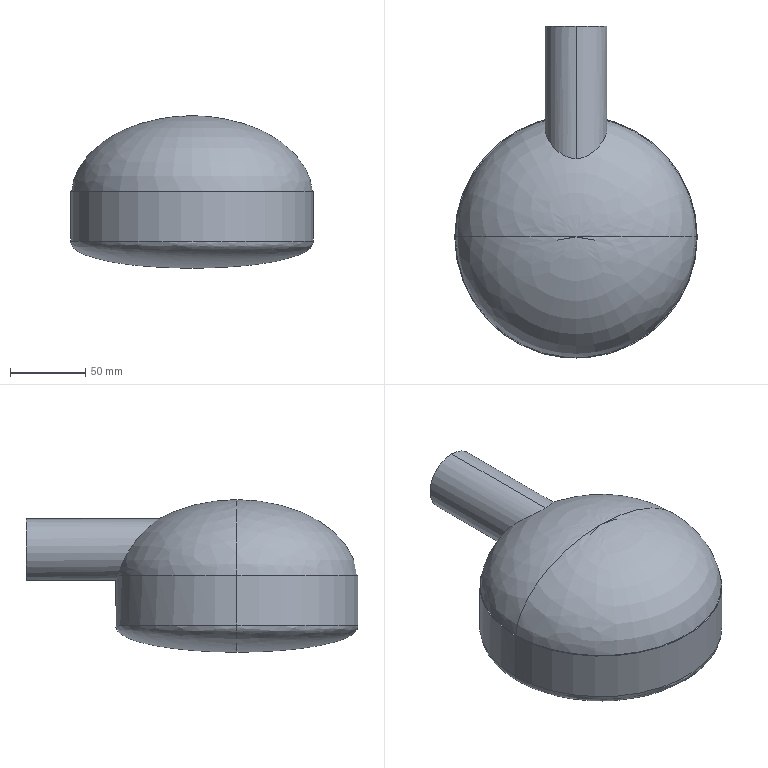Part | SolidWorks | 1 solid | 21 faces | box 161 x 220.5 x 101.1 mm | volume 223051 mm3 | cylinder 10 | spline 8 | plane 3 | commonest cylinder face diameters 35 x2 41 x2 154 x2 155 x2 161 x2